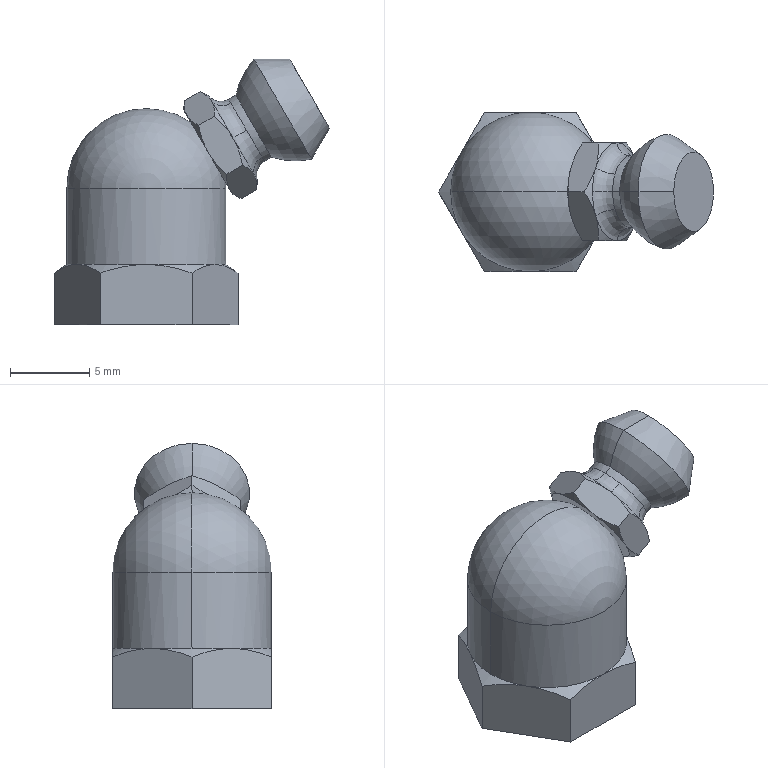Part | SolidWorks | features SplitBody 1 | 1 solid | 53 faces | box 17.303 x 10 x 16.688 mm | volume 1169 mm3 | cone 23 | plane 15 | torus 9 | cylinder 4 | sphere 2 | commonest cylinder face diameters 4.5 x2 10 x2